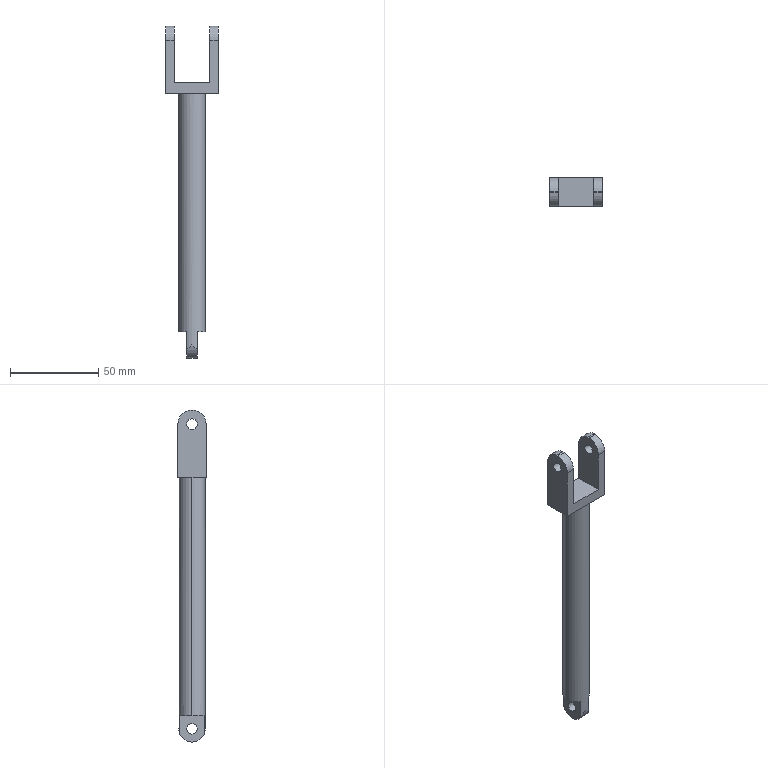Part | SolidWorks | features ICE 5, Extrusion 1 | 1 solid | 27 faces | box 30 x 16 x 188 mm | volume 32315 mm3 | plane 14 | cylinder 13 | commonest cylinder face diameters 6 x6 16 x4 15 x3
STEP:
#1=CARTESIAN_POINT('',(3.,0.,4.5));
#2=VERTEX_POINT('',#1);
#3=CARTESIAN_POINT('',(3.,0.,10.5));
#4=VERTEX_POINT('',#3);
#5=CARTESIAN_POINT('',(3.,0.,7.5));
#6=DIRECTION('',(-1.,0.,0.));
#7=DIRECTION('',(0.,0.,1.));
#8=AXIS2_PLACEMENT_3D('',#5,#6,#7);
#9=CIRCLE('',#8,3.);
#10=EDGE_CURVE('',#2,#4,#9,.T.);
#11=ORIENTED_EDGE('',*,*,#10,.F.);
#12=CARTESIAN_POINT('',(-3.,0.,4.5));
#13=VERTEX_POINT('',#12);
#14=CARTESIAN_POINT('',(15.001,0.,4.5));
#15=DIRECTION('',(-1.,0.,0.));
#16=VECTOR('',#15,1000.);
#17=LINE('',#14,#16);
#18=EDGE_CURVE('',#2,#13,#17,.T.);
#19=ORIENTED_EDGE('',*,*,#18,.T.);
#20=CARTESIAN_POINT('',(-3.,0.,10.5));
#21=VERTEX_POINT('',#20);
#22=CARTESIAN_POINT('',(-3.,0.,7.5));
#23=DIRECTION('',(1.,0.,0.));
#24=DIRECTION('',(0.,0.,-1.));
#25=AXIS2_PLACEMENT_3D('',#22,#23,#24);
#26=CIRCLE('',#25,3.);
#27=EDGE_CURVE('',#21,#13,#26,.T.);
#28=ORIENTED_EDGE('',*,*,#27,.F.);
#29=CARTESIAN_POINT('',(15.001,0.,10.5));
#30=DIRECTION('',(-1.,0.,0.));
#31=VECTOR('',#30,1000.);
#32=LINE('',#29,#31);
#33=EDGE_CURVE('',#4,#21,#32,.T.);
#34=ORIENTED_EDGE('',*,*,#33,.F.);
#35=EDGE_LOOP('',(#11,#19,#28,#34));
#36=FACE_OUTER_BOUND('',#35,.T.);
#37=CARTESIAN_POINT('',(15.001,0.,7.5));
#38=DIRECTION('',(-1.,0.,0.));
#39=DIRECTION('',(0.,0.,1.));
#40=AXIS2_PLACEMENT_3D('',#37,#38,#39);
#41=CYLINDRICAL_SURFACE('',#40,3.);
#42=ADVANCED_FACE('',(#36),#41,.F.);
#43=CARTESIAN_POINT('',(10.,-3.,180.015));
#44=VERTEX_POINT('',#43);
#45=CARTESIAN_POINT('',(10.,3.,180.015));
#46=VERTEX_POINT('',#45);
#47=CARTESIAN_POINT('',(10.,0.,180.015));
#48=DIRECTION('',(1.,0.,0.));
#49=DIRECTION('',(0.,1.,0.));
#50=AXIS2_PLACEMENT_3D('',#47,#48,#49);
#51=CIRCLE('',#50,3.);
#52=EDGE_CURVE('',#44,#46,#51,.T.);
#53=ORIENTED_EDGE('',*,*,#52,.F.);
#54=CARTESIAN_POINT('',(15.,-3.,180.015));
#55=VERTEX_POINT('',#54);
#56=CARTESIAN_POINT('',(-15.,-3.,180.015));
#57=DIRECTION('',(1.,0.,0.));
#58=VECTOR('',#57,1000.);
#59=LINE('',#56,#58);
#60=EDGE_CURVE('',#44,#55,#59,.T.);
#61=ORIENTED_EDGE('',*,*,#60,.T.);
#62=CARTESIAN_POINT('',(15.,3.,180.015));
#63=VERTEX_POINT('',#62);
#64=CARTESIAN_POINT('',(15.,0.,180.015));
#65=DIRECTION('',(-1.,0.,0.));
#66=DIRECTION('',(0.,-1.,0.));
#67=AXIS2_PLACEMENT_3D('',#64,#65,#66);
#68=CIRCLE('',#67,3.);
#69=EDGE_CURVE('',#63,#55,#68,.T.);
#70=ORIENTED_EDGE('',*,*,#69,.F.);
#71=CARTESIAN_POINT('',(-15.,3.,180.015));
#72=DIRECTION('',(1.,0.,0.));
#73=VECTOR('',#72,1000.);
#74=LINE('',#71,#73);
#75=EDGE_CURVE('',#46,#63,#74,.T.);
#76=ORIENTED_EDGE('',*,*,#75,.F.);
#77=EDGE_LOOP('',(#53,#61,#70,#76));
#78=FACE_OUTER_BOUND('',#77,.T.);
#79=CARTESIAN_POINT('',(-15.,0.,180.015));
#80=DIRECTION('',(1.,0.,0.));
#81=DIRECTION('',(0.,1.,0.));
#82=AXIS2_PLACEMENT_3D('',#79,#80,#81);
#83=CYLINDRICAL_SURFACE('',#82,3.);
#84=ADVANCED_FACE('',(#78),#83,.F.);
#85=CARTESIAN_POINT('',(-15.,-3.,180.015));
#86=VERTEX_POINT('',#85);
#87=CARTESIAN_POINT('',(-15.,3.,180.015));
#88=VERTEX_POINT('',#87);
#89=CARTESIAN_POINT('',(-15.,0.,180.015));
#90=DIRECTION('',(1.,0.,0.));
#91=DIRECTION('',(0.,1.,0.));
#92=AXIS2_PLACEMENT_3D('',#89,#90,#91);
#93=CIRCLE('',#92,3.);
#94=EDGE_CURVE('',#86,#88,#93,.T.);
#95=ORIENTED_EDGE('',*,*,#94,.F.);
#96=CARTESIAN_POINT('',(-10.,-3.,180.015));
#97=VERTEX_POINT('',#96);
#98=CARTESIAN_POINT('',(-15.,-3.,180.015));
#99=DIRECTION('',(1.,0.,0.));
#100=VECTOR('',#99,1000.);
#101=LINE('',#98,#100);
#102=EDGE_CURVE('',#86,#97,#101,.T.);
#103=ORIENTED_EDGE('',*,*,#102,.T.);
#104=CARTESIAN_POINT('',(-10.,3.,180.015));
#105=VERTEX_POINT('',#104);
#106=CARTESIAN_POINT('',(-10.,0.,180.015));
#107=DIRECTION('',(-1.,0.,0.));
#108=DIRECTION('',(0.,-1.,0.));
#109=AXIS2_PLACEMENT_3D('',#106,#107,#108);
#110=CIRCLE('',#109,3.);
#111=EDGE_CURVE('',#105,#97,#110,.T.);
#112=ORIENTED_EDGE('',*,*,#111,.F.);
#113=CARTESIAN_POINT('',(-15.,3.,180.015));
#114=DIRECTION('',(1.,0.,0.));
#115=VECTOR('',#114,1000.);
#116=LINE('',#113,#115);
#117=EDGE_CURVE('',#88,#105,#116,.T.);
#118=ORIENTED_EDGE('',*,*,#117,.F.);
#119=EDGE_LOOP('',(#95,#103,#112,#118));
#120=FACE_OUTER_BOUND('',#119,.T.);
#121=CARTESIAN_POINT('',(-15.,0.,180.015));
#122=DIRECTION('',(1.,0.,0.));
#123=DIRECTION('',(0.,1.,0.));
#124=AXIS2_PLACEMENT_3D('',#121,#122,#123);
#125=CYLINDRICAL_SURFACE('',#124,3.);
#126=ADVANCED_FACE('',(#120),#125,.F.);
#127=CARTESIAN_POINT('',(7.5,0.,150.));
#128=VERTEX_POINT('',#127);
#129=CARTESIAN_POINT('',(-7.5,0.,150.));
#130=VERTEX_POINT('',#129);
#131=CARTESIAN_POINT('',(0.,0.,150.));
#132=DIRECTION('',(0.,0.,1.));
#133=DIRECTION('',(1.,0.,0.));
#134=AXIS2_PLACEMENT_3D('',#131,#132,#133);
#135=CIRCLE('',#134,7.5);
#136=EDGE_CURVE('',#128,#130,#135,.T.);
#137=ORIENTED_EDGE('',*,*,#136,.F.);
#138=CARTESIAN_POINT('',(7.5,0.,15.));
#139=VERTEX_POINT('',#138);
#140=CARTESIAN_POINT('',(7.5,0.,150.));
#141=DIRECTION('',(0.,0.,-1.));
#142=VECTOR('',#141,1000.);
#143=LINE('',#140,#142);
#144=EDGE_CURVE('',#128,#139,#143,.T.);
#145=ORIENTED_EDGE('',*,*,#144,.T.);
#146=CARTESIAN_POINT('',(3.,6.874,15.));
#147=VERTEX_POINT('',#146);
#148=CARTESIAN_POINT('',(0.,0.,15.));
#149=DIRECTION('',(0.,0.,1.));
#150=DIRECTION('',(1.,0.,0.));
#151=AXIS2_PLACEMENT_3D('',#148,#149,#150);
#152=CIRCLE('',#151,7.5);
#153=EDGE_CURVE('',#139,#147,#152,.T.);
#154=ORIENTED_EDGE('',*,*,#153,.T.);
#155=CARTESIAN_POINT('',(3.,6.874,4.5));
#156=VERTEX_POINT('',#155);
#157=CARTESIAN_POINT('',(3.,6.874,150.));
#158=DIRECTION('',(0.,0.,-1.));
#159=VECTOR('',#158,1000.);
#160=LINE('',#157,#159);
#161=EDGE_CURVE('',#147,#156,#160,.T.);
#162=ORIENTED_EDGE('',*,*,#161,.T.);
#163=CARTESIAN_POINT('',(0.,7.5,7.5));
#164=VERTEX_POINT('',#163);
#165=CARTESIAN_POINT('',(3.,6.874,4.5));
#166=CARTESIAN_POINT('',(2.05,7.288,5.45));
#167=CARTESIAN_POINT('',(1.036,7.5,6.464));
#168=CARTESIAN_POINT('',(0.,7.5,7.5));
#169=(BOUNDED_CURVE()B_SPLINE_CURVE(3,(#165,#166,#167,#168),.UNSPECIFIED.,.F.,.T.)B_SPLINE_CURVE_WITH_KNOTS((4,4),(1.159,1.571),.UNSPECIFIED.)CURVE()GEOMETRIC_REPRESENTATION_ITEM()RATIONAL_B_SPLINE_CURVE((1.,0.9859,0.9859,1.))REPRESENTATION_ITEM(''));
#170=EDGE_CURVE('',#156,#164,#169,.T.);
#171=ORIENTED_EDGE('',*,*,#170,.T.);
#172=CARTESIAN_POINT('',(-3.,6.874,4.5));
#173=VERTEX_POINT('',#172);
#174=CARTESIAN_POINT('',(0.,7.5,7.5));
#175=CARTESIAN_POINT('',(-1.036,7.5,6.464));
#176=CARTESIAN_POINT('',(-2.05,7.288,5.45));
#177=CARTESIAN_POINT('',(-3.,6.874,4.5));
#178=(BOUNDED_CURVE()B_SPLINE_CURVE(3,(#174,#175,#176,#177),.UNSPECIFIED.,.F.,.T.)B_SPLINE_CURVE_WITH_KNOTS((4,4),(4.712,5.124),.UNSPECIFIED.)CURVE()GEOMETRIC_REPRESENTATION_ITEM()RATIONAL_B_SPLINE_CURVE((1.,0.9859,0.9859,1.))REPRESENTATION_ITEM(''));
#179=EDGE_CURVE('',#164,#173,#178,.T.);
#180=ORIENTED_EDGE('',*,*,#179,.T.);
#181=CARTESIAN_POINT('',(-3.,6.874,15.));
#182=VERTEX_POINT('',#181);
#183=CARTESIAN_POINT('',(-3.,6.874,150.));
#184=DIRECTION('',(0.,0.,1.));
#185=VECTOR('',#184,1000.);
#186=LINE('',#183,#185);
#187=EDGE_CURVE('',#173,#182,#186,.T.);
#188=ORIENTED_EDGE('',*,*,#187,.T.);
#189=CARTESIAN_POINT('',(-7.5,0.,15.));
#190=VERTEX_POINT('',#189);
#191=CARTESIAN_POINT('',(0.,0.,15.));
#192=DIRECTION('',(0.,0.,1.));
#193=DIRECTION('',(1.,0.,0.));
#194=AXIS2_PLACEMENT_3D('',#191,#192,#193);
#195=CIRCLE('',#194,7.5);
#196=EDGE_CURVE('',#182,#190,#195,.T.);
#197=ORIENTED_EDGE('',*,*,#196,.T.);
#198=CARTESIAN_POINT('',(-7.5,0.,150.));
#199=DIRECTION('',(0.,0.,-1.));
#200=VECTOR('',#199,1000.);
#201=LINE('',#198,#200);
#202=EDGE_CURVE('',#130,#190,#201,.T.);
#203=ORIENTED_EDGE('',*,*,#202,.F.);
#204=EDGE_LOOP('',(#137,#145,#154,#162,#171,#180,#188,#197,#203));
#205=FACE_OUTER_BOUND('',#204,.T.);
#206=CARTESIAN_POINT('',(0.,0.,150.));
#207=DIRECTION('',(0.,0.,-1.));
#208=DIRECTION('',(-1.,0.,0.));
#209=AXIS2_PLACEMENT_3D('',#206,#207,#208);
#210=CYLINDRICAL_SURFACE('',#209,7.5);
#211=ADVANCED_FACE('',(#205),#210,.T.);
#212=CARTESIAN_POINT('',(15.,-0.4894,188.));
#213=VERTEX_POINT('',#212);
#214=CARTESIAN_POINT('',(10.,-0.4894,188.));
#215=VERTEX_POINT('',#214);
#216=CARTESIAN_POINT('',(-15.,-0.4894,188.));
#217=DIRECTION('',(-1.,0.,0.));
#218=VECTOR('',#217,1000.);
#219=LINE('',#216,#218);
#220=EDGE_CURVE('',#213,#215,#219,.T.);
#221=ORIENTED_EDGE('',*,*,#220,.F.);
#222=CARTESIAN_POINT('',(15.,0.4894,188.));
#223=VERTEX_POINT('',#222);
#224=CARTESIAN_POINT('',(15.,8.,188.));
#225=DIRECTION('',(0.,1.,0.));
#226=VECTOR('',#225,1000.);
#227=LINE('',#224,#226);
#228=EDGE_CURVE('',#213,#223,#227,.T.);
#229=ORIENTED_EDGE('',*,*,#228,.T.);
#230=CARTESIAN_POINT('',(10.,0.4894,188.));
#231=VERTEX_POINT('',#230);
#232=CARTESIAN_POINT('',(-15.,0.4894,188.));
#233=DIRECTION('',(1.,0.,0.));
#234=VECTOR('',#233,1000.);
#235=LINE('',#232,#234);
#236=EDGE_CURVE('',#231,#223,#235,.T.);
#237=ORIENTED_EDGE('',*,*,#236,.F.);
#238=CARTESIAN_POINT('',(10.,0.,188.));
#239=DIRECTION('',(0.,1.,0.));
#240=VECTOR('',#239,1000.);
#241=LINE('',#238,#240);
#242=EDGE_CURVE('',#215,#231,#241,.T.);
#243=ORIENTED_EDGE('',*,*,#242,.F.);
#244=EDGE_LOOP('',(#221,#229,#237,#243));
#245=FACE_OUTER_BOUND('',#244,.T.);
#246=CARTESIAN_POINT('',(0.,0.,188.));
#247=DIRECTION('',(0.,0.,1.));
#248=DIRECTION('',(1.,0.,0.));
#249=AXIS2_PLACEMENT_3D('',#246,#247,#248);
#250=PLANE('',#249);
#251=ADVANCED_FACE('',(#245),#250,.T.);
#252=ORIENTED_EDGE('',*,*,#144,.F.);
#253=CARTESIAN_POINT('',(0.,0.,150.));
#254=DIRECTION('',(0.,0.,1.));
#255=DIRECTION('',(1.,0.,0.));
#256=AXIS2_PLACEMENT_3D('',#253,#254,#255);
#257=CIRCLE('',#256,7.5);
#258=EDGE_CURVE('',#130,#128,#257,.T.);
#259=ORIENTED_EDGE('',*,*,#258,.F.);
#260=ORIENTED_EDGE('',*,*,#202,.T.);
#261=CARTESIAN_POINT('',(-3.,-6.874,15.));
#262=VERTEX_POINT('',#261);
#263=CARTESIAN_POINT('',(0.,0.,15.));
#264=DIRECTION('',(0.,0.,1.));
#265=DIRECTION('',(1.,0.,0.));
#266=AXIS2_PLACEMENT_3D('',#263,#264,#265);
#267=CIRCLE('',#266,7.5);
#268=EDGE_CURVE('',#190,#262,#267,.T.);
#269=ORIENTED_EDGE('',*,*,#268,.T.);
#270=CARTESIAN_POINT('',(-3.,-6.874,4.5));
#271=VERTEX_POINT('',#270);
#272=CARTESIAN_POINT('',(-3.,-6.874,150.));
#273=DIRECTION('',(0.,0.,-1.));
#274=VECTOR('',#273,1000.);
#275=LINE('',#272,#274);
#276=EDGE_CURVE('',#262,#271,#275,.T.);
#277=ORIENTED_EDGE('',*,*,#276,.T.);
#278=CARTESIAN_POINT('',(0.,-7.5,7.5));
#279=VERTEX_POINT('',#278);
#280=CARTESIAN_POINT('',(-3.,-6.874,4.5));
#281=CARTESIAN_POINT('',(-2.05,-7.288,5.45));
#282=CARTESIAN_POINT('',(-1.036,-7.5,6.464));
#283=CARTESIAN_POINT('',(0.,-7.5,7.5));
#284=(BOUNDED_CURVE()B_SPLINE_CURVE(3,(#280,#281,#282,#283),.UNSPECIFIED.,.F.,.T.)B_SPLINE_CURVE_WITH_KNOTS((4,4),(1.159,1.571),.UNSPECIFIED.)CURVE()GEOMETRIC_REPRESENTATION_ITEM()RATIONAL_B_SPLINE_CURVE((1.,0.9859,0.9859,1.))REPRESENTATION_ITEM(''));
#285=EDGE_CURVE('',#271,#279,#284,.T.);
#286=ORIENTED_EDGE('',*,*,#285,.T.);
#287=CARTESIAN_POINT('',(3.,-6.874,4.5));
#288=VERTEX_POINT('',#287);
#289=CARTESIAN_POINT('',(0.,-7.5,7.5));
#290=CARTESIAN_POINT('',(1.036,-7.5,6.464));
#291=CARTESIAN_POINT('',(2.05,-7.288,5.45));
#292=CARTESIAN_POINT('',(3.,-6.874,4.5));
#293=(BOUNDED_CURVE()B_SPLINE_CURVE(3,(#289,#290,#291,#292),.UNSPECIFIED.,.F.,.T.)B_SPLINE_CURVE_WITH_KNOTS((4,4),(4.712,5.124),.UNSPECIFIED.)CURVE()GEOMETRIC_REPRESENTATION_ITEM()RATIONAL_B_SPLINE_CURVE((1.,0.9859,0.9859,1.))REPRESENTATION_ITEM(''));
#294=EDGE_CURVE('',#279,#288,#293,.T.);
#295=ORIENTED_EDGE('',*,*,#294,.T.);
#296=CARTESIAN_POINT('',(3.,-6.874,15.));
#297=VERTEX_POINT('',#296);
#298=CARTESIAN_POINT('',(3.,-6.874,150.));
#299=DIRECTION('',(0.,0.,1.));
#300=VECTOR('',#299,1000.);
#301=LINE('',#298,#300);
#302=EDGE_CURVE('',#288,#297,#301,.T.);
#303=ORIENTED_EDGE('',*,*,#302,.T.);
#304=CARTESIAN_POINT('',(0.,0.,15.));
#305=DIRECTION('',(0.,0.,1.));
#306=DIRECTION('',(1.,0.,0.));
#307=AXIS2_PLACEMENT_3D('',#304,#305,#306);
#308=CIRCLE('',#307,7.5);
#309=EDGE_CURVE('',#297,#139,#308,.T.);
#310=ORIENTED_EDGE('',*,*,#309,.T.);
#311=EDGE_LOOP('',(#252,#259,#260,#269,#277,#286,#295,#303,#310));
#312=FACE_OUTER_BOUND('',#311,.T.);
#313=CARTESIAN_POINT('',(0.,0.,150.));
#314=DIRECTION('',(0.,0.,-1.));
#315=DIRECTION('',(-1.,0.,0.));
#316=AXIS2_PLACEMENT_3D('',#313,#314,#315);
#317=CYLINDRICAL_SURFACE('',#316,7.5);
#318=ADVANCED_FACE('',(#312),#317,.T.);
#319=ORIENTED_EDGE('',*,*,#69,.T.);
#320=CARTESIAN_POINT('',(15.,0.,180.015));
#321=DIRECTION('',(-1.,0.,0.));
#322=DIRECTION('',(0.,-1.,0.));
#323=AXIS2_PLACEMENT_3D('',#320,#321,#322);
#324=CIRCLE('',#323,3.);
#325=EDGE_CURVE('',#55,#63,#324,.T.);
#326=ORIENTED_EDGE('',*,*,#325,.T.);
#327=EDGE_LOOP('',(#319,#326));
#328=FACE_BOUND('',#327,.T.);
#329=CARTESIAN_POINT('',(15.,8.,180.015));
#330=VERTEX_POINT('',#329);
#331=CARTESIAN_POINT('',(15.,8.,150.));
#332=VERTEX_POINT('',#331);
#333=CARTESIAN_POINT('',(15.,8.,188.));
#334=DIRECTION('',(0.,0.,-1.));
#335=VECTOR('',#334,1000.);
#336=LINE('',#333,#335);
#337=EDGE_CURVE('',#330,#332,#336,.T.);
#338=ORIENTED_EDGE('',*,*,#337,.F.);
#339=CARTESIAN_POINT('',(15.,0.,180.015));
#340=DIRECTION('',(1.,0.,0.));
#341=DIRECTION('',(0.,-1.,0.));
#342=AXIS2_PLACEMENT_3D('',#339,#340,#341);
#343=CIRCLE('',#342,8.);
#344=EDGE_CURVE('',#330,#223,#343,.T.);
#345=ORIENTED_EDGE('',*,*,#344,.T.);
#346=ORIENTED_EDGE('',*,*,#228,.F.);
#347=CARTESIAN_POINT('',(15.,-8.,180.015));
#348=VERTEX_POINT('',#347);
#349=CARTESIAN_POINT('',(15.,0.,180.015));
#350=DIRECTION('',(1.,0.,0.));
#351=DIRECTION('',(0.,-1.,0.));
#352=AXIS2_PLACEMENT_3D('',#349,#350,#351);
#353=CIRCLE('',#352,8.);
#354=EDGE_CURVE('',#213,#348,#353,.T.);
#355=ORIENTED_EDGE('',*,*,#354,.T.);
#356=CARTESIAN_POINT('',(15.,-8.,150.));
#357=VERTEX_POINT('',#356);
#358=CARTESIAN_POINT('',(15.,-8.,188.));
#359=DIRECTION('',(0.,0.,-1.));
#360=VECTOR('',#359,1000.);
#361=LINE('',#358,#360);
#362=EDGE_CURVE('',#348,#357,#361,.T.);
#363=ORIENTED_EDGE('',*,*,#362,.T.);
#364=CARTESIAN_POINT('',(15.,8.,150.));
#365=DIRECTION('',(0.,1.,0.));
#366=VECTOR('',#365,1000.);
#367=LINE('',#364,#366);
#368=EDGE_CURVE('',#357,#332,#367,.T.);
#369=ORIENTED_EDGE('',*,*,#368,.T.);
#370=EDGE_LOOP('',(#338,#345,#346,#355,#363,#369));
#371=FACE_OUTER_BOUND('',#370,.T.);
#372=CARTESIAN_POINT('',(15.,8.,188.));
#373=DIRECTION('',(-1.,0.,0.));
#374=DIRECTION('',(0.,-1.,0.));
#375=AXIS2_PLACEMENT_3D('',#372,#373,#374);
#376=PLANE('',#375);
#377=ADVANCED_FACE('',(#328,#371),#376,.F.);
#378=CARTESIAN_POINT('',(-15.,8.,180.015));
#379=VERTEX_POINT('',#378);
#380=CARTESIAN_POINT('',(-15.,8.,150.));
#381=VERTEX_POINT('',#380);
#382=CARTESIAN_POINT('',(-15.,8.,188.));
#383=DIRECTION('',(0.,0.,-1.));
#384=VECTOR('',#383,1000.);
#385=LINE('',#382,#384);
#386=EDGE_CURVE('',#379,#381,#385,.T.);
#387=ORIENTED_EDGE('',*,*,#386,.F.);
#388=CARTESIAN_POINT('',(-10.,8.,180.015));
#389=VERTEX_POINT('',#388);
#390=CARTESIAN_POINT('',(-15.,8.,180.015));
#391=DIRECTION('',(1.,0.,0.));
#392=VECTOR('',#391,1000.);
#393=LINE('',#390,#392);
#394=EDGE_CURVE('',#379,#389,#393,.T.);
#395=ORIENTED_EDGE('',*,*,#394,.T.);
#396=CARTESIAN_POINT('',(-10.,8.,156.));
#397=VERTEX_POINT('',#396);
#398=CARTESIAN_POINT('',(-10.,8.,188.));
#399=DIRECTION('',(0.,0.,-1.));
#400=VECTOR('',#399,1000.);
#401=LINE('',#398,#400);
#402=EDGE_CURVE('',#389,#397,#401,.T.);
#403=ORIENTED_EDGE('',*,*,#402,.T.);
#404=CARTESIAN_POINT('',(10.,8.,156.));
#405=VERTEX_POINT('',#404);
#406=CARTESIAN_POINT('',(-15.,8.,156.));
#407=DIRECTION('',(-1.,0.,0.));
#408=VECTOR('',#407,1000.);
#409=LINE('',#406,#408);
#410=EDGE_CURVE('',#405,#397,#409,.T.);
#411=ORIENTED_EDGE('',*,*,#410,.F.);
#412=CARTESIAN_POINT('',(10.,8.,180.015));
#413=VERTEX_POINT('',#412);
#414=CARTESIAN_POINT('',(10.,8.,188.));
#415=DIRECTION('',(0.,0.,1.));
#416=VECTOR('',#415,1000.);
#417=LINE('',#414,#416);
#418=EDGE_CURVE('',#405,#413,#417,.T.);
#419=ORIENTED_EDGE('',*,*,#418,.T.);
#420=CARTESIAN_POINT('',(-15.,8.,180.015));
#421=DIRECTION('',(1.,0.,0.));
#422=VECTOR('',#421,1000.);
#423=LINE('',#420,#422);
#424=EDGE_CURVE('',#413,#330,#423,.T.);
#425=ORIENTED_EDGE('',*,*,#424,.T.);
#426=ORIENTED_EDGE('',*,*,#337,.T.);
#427=CARTESIAN_POINT('',(-15.,8.,150.));
#428=DIRECTION('',(-1.,0.,0.));
#429=VECTOR('',#428,1000.);
#430=LINE('',#427,#429);
#431=EDGE_CURVE('',#332,#381,#430,.T.);
#432=ORIENTED_EDGE('',*,*,#431,.T.);
#433=EDGE_LOOP('',(#387,#395,#403,#411,#419,#425,#426,#432));
#434=FACE_OUTER_BOUND('',#433,.T.);
#435=CARTESIAN_POINT('',(-15.,8.,188.));
#436=DIRECTION('',(0.,-1.,0.));
#437=DIRECTION('',(0.,0.,-1.));
#438=AXIS2_PLACEMENT_3D('',#435,#436,#437);
#439=PLANE('',#438);
#440=ADVANCED_FACE('',(#434),#439,.F.);
#441=CARTESIAN_POINT('',(-15.,0.,180.015));
#442=DIRECTION('',(1.,0.,0.));
#443=DIRECTION('',(0.,1.,0.));
#444=AXIS2_PLACEMENT_3D('',#441,#442,#443);
#445=CIRCLE('',#444,3.);
#446=EDGE_CURVE('',#88,#86,#445,.T.);
#447=ORIENTED_EDGE('',*,*,#446,.T.);
#448=ORIENTED_EDGE('',*,*,#94,.T.);
#449=EDGE_LOOP('',(#447,#448));
#450=FACE_BOUND('',#449,.T.);
#451=CARTESIAN_POINT('',(-15.,-8.,180.015));
#452=VERTEX_POINT('',#451);
#453=CARTESIAN_POINT('',(-15.,-8.,150.));
#454=VERTEX_POINT('',#453);
#455=CARTESIAN_POINT('',(-15.,-8.,188.));
#456=DIRECTION('',(0.,0.,-1.));
#457=VECTOR('',#456,1000.);
#458=LINE('',#455,#457);
#459=EDGE_CURVE('',#452,#454,#458,.T.);
#460=ORIENTED_EDGE('',*,*,#459,.F.);
#461=CARTESIAN_POINT('',(-15.,-0.4894,188.));
#462=VERTEX_POINT('',#461);
#463=CARTESIAN_POINT('',(-15.,0.,180.015));
#464=DIRECTION('',(-1.,0.,0.));
#465=DIRECTION('',(0.,1.,0.));
#466=AXIS2_PLACEMENT_3D('',#463,#464,#465);
#467=CIRCLE('',#466,8.);
#468=EDGE_CURVE('',#452,#462,#467,.T.);
#469=ORIENTED_EDGE('',*,*,#468,.T.);
#470=CARTESIAN_POINT('',(-15.,0.4894,188.));
#471=VERTEX_POINT('',#470);
#472=CARTESIAN_POINT('',(-15.,8.,188.));
#473=DIRECTION('',(0.,-1.,0.));
#474=VECTOR('',#473,1000.);
#475=LINE('',#472,#474);
#476=EDGE_CURVE('',#471,#462,#475,.T.);
#477=ORIENTED_EDGE('',*,*,#476,.F.);
#478=CARTESIAN_POINT('',(-15.,0.,180.015));
#479=DIRECTION('',(-1.,0.,0.));
#480=DIRECTION('',(0.,1.,0.));
#481=AXIS2_PLACEMENT_3D('',#478,#479,#480);
#482=CIRCLE('',#481,8.);
#483=EDGE_CURVE('',#471,#379,#482,.T.);
#484=ORIENTED_EDGE('',*,*,#483,.T.);
#485=ORIENTED_EDGE('',*,*,#386,.T.);
#486=CARTESIAN_POINT('',(-15.,8.,150.));
#487=DIRECTION('',(0.,-1.,0.));
#488=VECTOR('',#487,1000.);
#489=LINE('',#486,#488);
#490=EDGE_CURVE('',#381,#454,#489,.T.);
#491=ORIENTED_EDGE('',*,*,#490,.T.);
#492=EDGE_LOOP('',(#460,#469,#477,#484,#485,#491));
#493=FACE_OUTER_BOUND('',#492,.T.);
#494=CARTESIAN_POINT('',(-15.,8.,188.));
#495=DIRECTION('',(1.,0.,0.));
#496=DIRECTION('',(0.,1.,0.));
#497=AXIS2_PLACEMENT_3D('',#494,#495,#496);
#498=PLANE('',#497);
#499=ADVANCED_FACE('',(#450,#493),#498,.F.);
#500=ORIENTED_EDGE('',*,*,#362,.F.);
#501=CARTESIAN_POINT('',(10.,-8.,180.015));
#502=VERTEX_POINT('',#501);
#503=CARTESIAN_POINT('',(-15.,-8.,180.015));
#504=DIRECTION('',(1.,0.,0.));
#505=VECTOR('',#504,1000.);
#506=LINE('',#503,#505);
#507=EDGE_CURVE('',#502,#348,#506,.T.);
#508=ORIENTED_EDGE('',*,*,#507,.F.);
#509=CARTESIAN_POINT('',(10.,-8.,156.));
#510=VERTEX_POINT('',#509);
#511=CARTESIAN_POINT('',(10.,-8.,188.));
#512=DIRECTION('',(0.,0.,-1.));
#513=VECTOR('',#512,1000.);
#514=LINE('',#511,#513);
#515=EDGE_CURVE('',#502,#510,#514,.T.);
#516=ORIENTED_EDGE('',*,*,#515,.T.);
#517=CARTESIAN_POINT('',(-10.,-8.,156.));
#518=VERTEX_POINT('',#517);
#519=CARTESIAN_POINT('',(-15.,-8.,156.));
#520=DIRECTION('',(1.,0.,0.));
#521=VECTOR('',#520,1000.);
#522=LINE('',#519,#521);
#523=EDGE_CURVE('',#518,#510,#522,.T.);
#524=ORIENTED_EDGE('',*,*,#523,.F.);
#525=CARTESIAN_POINT('',(-10.,-8.,180.015));
#526=VERTEX_POINT('',#525);
#527=CARTESIAN_POINT('',(-10.,-8.,188.));
#528=DIRECTION('',(0.,0.,1.));
#529=VECTOR('',#528,1000.);
#530=LINE('',#527,#529);
#531=EDGE_CURVE('',#518,#526,#530,.T.);
#532=ORIENTED_EDGE('',*,*,#531,.T.);
#533=CARTESIAN_POINT('',(-15.,-8.,180.015));
#534=DIRECTION('',(1.,0.,0.));
#535=VECTOR('',#534,1000.);
#536=LINE('',#533,#535);
#537=EDGE_CURVE('',#452,#526,#536,.T.);
#538=ORIENTED_EDGE('',*,*,#537,.F.);
#539=ORIENTED_EDGE('',*,*,#459,.T.);
#540=CARTESIAN_POINT('',(-15.,-8.,150.));
#541=DIRECTION('',(1.,0.,0.));
#542=VECTOR('',#541,1000.);
#543=LINE('',#540,#542);
#544=EDGE_CURVE('',#454,#357,#543,.T.);
#545=ORIENTED_EDGE('',*,*,#544,.T.);
#546=EDGE_LOOP('',(#500,#508,#516,#524,#532,#538,#539,#545));
#547=FACE_OUTER_BOUND('',#546,.T.);
#548=CARTESIAN_POINT('',(-15.,-8.,188.));
#549=DIRECTION('',(0.,1.,0.));
#550=DIRECTION('',(0.,0.,1.));
#551=AXIS2_PLACEMENT_3D('',#548,#549,#550);
#552=PLANE('',#551);
#553=ADVANCED_FACE('',(#547),#552,.F.);
#554=CARTESIAN_POINT('',(-10.,-0.4894,188.));
#555=VERTEX_POINT('',#554);
#556=CARTESIAN_POINT('',(-15.,-0.4894,188.));
#557=DIRECTION('',(-1.,0.,0.));
#558=VECTOR('',#557,1000.);
#559=LINE('',#556,#558);
#560=EDGE_CURVE('',#555,#462,#559,.T.);
#561=ORIENTED_EDGE('',*,*,#560,.F.);
#562=CARTESIAN_POINT('',(-10.,0.4894,188.));
#563=VERTEX_POINT('',#562);
#564=CARTESIAN_POINT('',(-10.,0.,188.));
#565=DIRECTION('',(0.,-1.,0.));
#566=VECTOR('',#565,1000.);
#567=LINE('',#564,#566);
#568=EDGE_CURVE('',#563,#555,#567,.T.);
#569=ORIENTED_EDGE('',*,*,#568,.F.);
#570=CARTESIAN_POINT('',(-15.,0.4894,188.));
#571=DIRECTION('',(1.,0.,0.));
#572=VECTOR('',#571,1000.);
#573=LINE('',#570,#572);
#574=EDGE_CURVE('',#471,#563,#573,.T.);
#575=ORIENTED_EDGE('',*,*,#574,.F.);
#576=ORIENTED_EDGE('',*,*,#476,.T.);
#577=EDGE_LOOP('',(#561,#569,#575,#576));
#578=FACE_OUTER_BOUND('',#577,.T.);
#579=CARTESIAN_POINT('',(0.,0.,188.));
#580=DIRECTION('',(0.,0.,1.));
#581=DIRECTION('',(1.,0.,0.));
#582=AXIS2_PLACEMENT_3D('',#579,#580,#581);
#583=PLANE('',#582);
#584=ADVANCED_FACE('',(#578),#583,.T.);
#585=ORIENTED_EDGE('',*,*,#258,.T.);
#586=ORIENTED_EDGE('',*,*,#136,.T.);
#587=EDGE_LOOP('',(#585,#586));
#588=FACE_BOUND('',#587,.T.);
#589=ORIENTED_EDGE('',*,*,#368,.F.);
#590=ORIENTED_EDGE('',*,*,#544,.F.);
#591=ORIENTED_EDGE('',*,*,#490,.F.);
#592=ORIENTED_EDGE('',*,*,#431,.F.);
#593=EDGE_LOOP('',(#589,#590,#591,#592));
#594=FACE_OUTER_BOUND('',#593,.T.);
#595=CARTESIAN_POINT('',(0.,0.,150.));
#596=DIRECTION('',(0.,0.,1.));
#597=DIRECTION('',(1.,0.,0.));
#598=AXIS2_PLACEMENT_3D('',#595,#596,#597);
#599=PLANE('',#598);
#600=ADVANCED_FACE('',(#588,#594),#599,.F.);
#601=ORIENTED_EDGE('',*,*,#410,.T.);
#602=CARTESIAN_POINT('',(-10.,9.679,156.));
#603=DIRECTION('',(0.,-1.,0.));
#604=VECTOR('',#603,1000.);
#605=LINE('',#602,#604);
#606=EDGE_CURVE('',#397,#518,#605,.T.);
#607=ORIENTED_EDGE('',*,*,#606,.T.);
#608=ORIENTED_EDGE('',*,*,#523,.T.);
#609=CARTESIAN_POINT('',(10.,9.679,156.));
#610=DIRECTION('',(0.,1.,0.));
#611=VECTOR('',#610,1000.);
#612=LINE('',#609,#611);
#613=EDGE_CURVE('',#510,#405,#612,.T.);
#614=ORIENTED_EDGE('',*,*,#613,.T.);
#615=EDGE_LOOP('',(#601,#607,#608,#614));
#616=FACE_OUTER_BOUND('',#615,.T.);
#617=CARTESIAN_POINT('',(0.,0.,156.));
#618=DIRECTION('',(0.,0.,1.));
#619=DIRECTION('',(1.,0.,0.));
#620=AXIS2_PLACEMENT_3D('',#617,#618,#619);
#621=PLANE('',#620);
#622=ADVANCED_FACE('',(#616),#621,.T.);
#623=CARTESIAN_POINT('',(10.,0.,180.015));
#624=DIRECTION('',(1.,0.,0.));
#625=DIRECTION('',(0.,1.,0.));
#626=AXIS2_PLACEMENT_3D('',#623,#624,#625);
#627=CIRCLE('',#626,3.);
#628=EDGE_CURVE('',#46,#44,#627,.T.);
#629=ORIENTED_EDGE('',*,*,#628,.T.);
#630=ORIENTED_EDGE('',*,*,#52,.T.);
#631=EDGE_LOOP('',(#629,#630));
#632=FACE_BOUND('',#631,.T.);
#633=ORIENTED_EDGE('',*,*,#515,.F.);
#634=CARTESIAN_POINT('',(10.,0.,180.015));
#635=DIRECTION('',(-1.,0.,0.));
#636=DIRECTION('',(0.,1.,0.));
#637=AXIS2_PLACEMENT_3D('',#634,#635,#636);
#638=CIRCLE('',#637,8.);
#639=EDGE_CURVE('',#502,#215,#638,.T.);
#640=ORIENTED_EDGE('',*,*,#639,.T.);
#641=ORIENTED_EDGE('',*,*,#242,.T.);
#642=CARTESIAN_POINT('',(10.,0.,180.015));
#643=DIRECTION('',(-1.,0.,0.));
#644=DIRECTION('',(0.,1.,0.));
#645=AXIS2_PLACEMENT_3D('',#642,#643,#644);
#646=CIRCLE('',#645,8.);
#647=EDGE_CURVE('',#231,#413,#646,.T.);
#648=ORIENTED_EDGE('',*,*,#647,.T.);
#649=ORIENTED_EDGE('',*,*,#418,.F.);
#650=ORIENTED_EDGE('',*,*,#613,.F.);
#651=EDGE_LOOP('',(#633,#640,#641,#648,#649,#650));
#652=FACE_OUTER_BOUND('',#651,.T.);
#653=CARTESIAN_POINT('',(10.,9.679,156.));
#654=DIRECTION('',(1.,0.,0.));
#655=DIRECTION('',(0.,1.,0.));
#656=AXIS2_PLACEMENT_3D('',#653,#654,#655);
#657=PLANE('',#656);
#658=ADVANCED_FACE('',(#632,#652),#657,.F.);
#659=ORIENTED_EDGE('',*,*,#111,.T.);
#660=CARTESIAN_POINT('',(-10.,0.,180.015));
#661=DIRECTION('',(-1.,0.,0.));
#662=DIRECTION('',(0.,-1.,0.));
#663=AXIS2_PLACEMENT_3D('',#660,#661,#662);
#664=CIRCLE('',#663,3.);
#665=EDGE_CURVE('',#97,#105,#664,.T.);
#666=ORIENTED_EDGE('',*,*,#665,.T.);
#667=EDGE_LOOP('',(#659,#666));
#668=FACE_BOUND('',#667,.T.);
#669=ORIENTED_EDGE('',*,*,#402,.F.);
#670=CARTESIAN_POINT('',(-10.,0.,180.015));
#671=DIRECTION('',(1.,0.,0.));
#672=DIRECTION('',(0.,-1.,0.));
#673=AXIS2_PLACEMENT_3D('',#670,#671,#672);
#674=CIRCLE('',#673,8.);
#675=EDGE_CURVE('',#389,#563,#674,.T.);
#676=ORIENTED_EDGE('',*,*,#675,.T.);
#677=ORIENTED_EDGE('',*,*,#568,.T.);
#678=CARTESIAN_POINT('',(-10.,0.,180.015));
#679=DIRECTION('',(1.,0.,0.));
#680=DIRECTION('',(0.,-1.,0.));
#681=AXIS2_PLACEMENT_3D('',#678,#679,#680);
#682=CIRCLE('',#681,8.);
#683=EDGE_CURVE('',#555,#526,#682,.T.);
#684=ORIENTED_EDGE('',*,*,#683,.T.);
#685=ORIENTED_EDGE('',*,*,#531,.F.);
#686=ORIENTED_EDGE('',*,*,#606,.F.);
#687=EDGE_LOOP('',(#669,#676,#677,#684,#685,#686));
#688=FACE_OUTER_BOUND('',#687,.T.);
#689=CARTESIAN_POINT('',(-10.,9.679,156.));
#690=DIRECTION('',(-1.,0.,0.));
#691=DIRECTION('',(0.,-1.,0.));
#692=AXIS2_PLACEMENT_3D('',#689,#690,#691);
#693=PLANE('',#692);
#694=ADVANCED_FACE('',(#668,#688),#693,.F.);
#695=ORIENTED_EDGE('',*,*,#102,.F.);
#696=ORIENTED_EDGE('',*,*,#446,.F.);
#697=ORIENTED_EDGE('',*,*,#117,.T.);
#698=ORIENTED_EDGE('',*,*,#665,.F.);
#699=EDGE_LOOP('',(#695,#696,#697,#698));
#700=FACE_OUTER_BOUND('',#699,.T.);
#701=CARTESIAN_POINT('',(-15.,0.,180.015));
#702=DIRECTION('',(1.,0.,0.));
#703=DIRECTION('',(0.,1.,0.));
#704=AXIS2_PLACEMENT_3D('',#701,#702,#703);
#705=CYLINDRICAL_SURFACE('',#704,3.);
#706=ADVANCED_FACE('',(#700),#705,.F.);
#707=ORIENTED_EDGE('',*,*,#560,.T.);
#708=ORIENTED_EDGE('',*,*,#468,.F.);
#709=ORIENTED_EDGE('',*,*,#537,.T.);
#710=ORIENTED_EDGE('',*,*,#683,.F.);
#711=EDGE_LOOP('',(#707,#708,#709,#710));
#712=FACE_OUTER_BOUND('',#711,.T.);
#713=CARTESIAN_POINT('',(-15.,0.,180.015));
#714=DIRECTION('',(1.,0.,0.));
#715=DIRECTION('',(0.,1.,0.));
#716=AXIS2_PLACEMENT_3D('',#713,#714,#715);
#717=CYLINDRICAL_SURFACE('',#716,8.);
#718=ADVANCED_FACE('',(#712),#717,.T.);
#719=ORIENTED_EDGE('',*,*,#574,.T.);
#720=ORIENTED_EDGE('',*,*,#675,.F.);
#721=ORIENTED_EDGE('',*,*,#394,.F.);
#722=ORIENTED_EDGE('',*,*,#483,.F.);
#723=EDGE_LOOP('',(#719,#720,#721,#722));
#724=FACE_OUTER_BOUND('',#723,.T.);
#725=CARTESIAN_POINT('',(-15.,0.,180.015));
#726=DIRECTION('',(1.,0.,0.));
#727=DIRECTION('',(0.,1.,0.));
#728=AXIS2_PLACEMENT_3D('',#725,#726,#727);
#729=CYLINDRICAL_SURFACE('',#728,8.);
#730=ADVANCED_FACE('',(#724),#729,.T.);
#731=ORIENTED_EDGE('',*,*,#60,.F.);
#732=ORIENTED_EDGE('',*,*,#628,.F.);
#733=ORIENTED_EDGE('',*,*,#75,.T.);
#734=ORIENTED_EDGE('',*,*,#325,.F.);
#735=EDGE_LOOP('',(#731,#732,#733,#734));
#736=FACE_OUTER_BOUND('',#735,.T.);
#737=CARTESIAN_POINT('',(-15.,0.,180.015));
#738=DIRECTION('',(1.,0.,0.));
#739=DIRECTION('',(0.,1.,0.));
#740=AXIS2_PLACEMENT_3D('',#737,#738,#739);
#741=CYLINDRICAL_SURFACE('',#740,3.);
#742=ADVANCED_FACE('',(#736),#741,.F.);
#743=ORIENTED_EDGE('',*,*,#424,.F.);
#744=ORIENTED_EDGE('',*,*,#647,.F.);
#745=ORIENTED_EDGE('',*,*,#236,.T.);
#746=ORIENTED_EDGE('',*,*,#344,.F.);
#747=EDGE_LOOP('',(#743,#744,#745,#746));
#748=FACE_OUTER_BOUND('',#747,.T.);
#749=CARTESIAN_POINT('',(-15.,0.,180.015));
#750=DIRECTION('',(1.,0.,0.));
#751=DIRECTION('',(0.,1.,0.));
#752=AXIS2_PLACEMENT_3D('',#749,#750,#751);
#753=CYLINDRICAL_SURFACE('',#752,8.);
#754=ADVANCED_FACE('',(#748),#753,.T.);
#755=ORIENTED_EDGE('',*,*,#220,.T.);
#756=ORIENTED_EDGE('',*,*,#639,.F.);
#757=ORIENTED_EDGE('',*,*,#507,.T.);
#758=ORIENTED_EDGE('',*,*,#354,.F.);
#759=EDGE_LOOP('',(#755,#756,#757,#758));
#760=FACE_OUTER_BOUND('',#759,.T.);
#761=CARTESIAN_POINT('',(-15.,0.,180.015));
#762=DIRECTION('',(1.,0.,0.));
#763=DIRECTION('',(0.,1.,0.));
#764=AXIS2_PLACEMENT_3D('',#761,#762,#763);
#765=CYLINDRICAL_SURFACE('',#764,8.);
#766=ADVANCED_FACE('',(#760),#765,.T.);
#767=CARTESIAN_POINT('',(3.,-8.001,15.));
#768=DIRECTION('',(0.,1.,0.));
#769=VECTOR('',#768,1000.);
#770=LINE('',#767,#769);
#771=EDGE_CURVE('',#297,#147,#770,.T.);
#772=ORIENTED_EDGE('',*,*,#771,.T.);
#773=ORIENTED_EDGE('',*,*,#153,.F.);
#774=ORIENTED_EDGE('',*,*,#309,.F.);
#775=EDGE_LOOP('',(#772,#773,#774));
#776=FACE_OUTER_BOUND('',#775,.T.);
#777=CARTESIAN_POINT('',(22.943,-8.001,15.));
#778=DIRECTION('',(0.,0.,1.));
#779=DIRECTION('',(1.,0.,0.));
#780=AXIS2_PLACEMENT_3D('',#777,#778,#779);
#781=PLANE('',#780);
#782=ADVANCED_FACE('',(#776),#781,.F.);
#783=CARTESIAN_POINT('',(3.,0.,7.5));
#784=DIRECTION('',(-1.,0.,0.));
#785=DIRECTION('',(0.,0.,1.));
#786=AXIS2_PLACEMENT_3D('',#783,#784,#785);
#787=CIRCLE('',#786,3.);
#788=EDGE_CURVE('',#4,#2,#787,.T.);
#789=ORIENTED_EDGE('',*,*,#788,.T.);
#790=ORIENTED_EDGE('',*,*,#10,.T.);
#791=EDGE_LOOP('',(#789,#790));
#792=FACE_BOUND('',#791,.T.);
#793=ORIENTED_EDGE('',*,*,#302,.F.);
#794=CARTESIAN_POINT('',(3.,0.,7.5));
#795=DIRECTION('',(1.,0.,0.));
#796=DIRECTION('',(0.,0.,1.));
#797=AXIS2_PLACEMENT_3D('',#794,#795,#796);
#798=CIRCLE('',#797,7.5);
#799=EDGE_CURVE('',#288,#156,#798,.T.);
#800=ORIENTED_EDGE('',*,*,#799,.T.);
#801=ORIENTED_EDGE('',*,*,#161,.F.);
#802=ORIENTED_EDGE('',*,*,#771,.F.);
#803=EDGE_LOOP('',(#793,#800,#801,#802));
#804=FACE_OUTER_BOUND('',#803,.T.);
#805=CARTESIAN_POINT('',(3.,-8.001,15.));
#806=DIRECTION('',(-1.,0.,0.));
#807=DIRECTION('',(0.,0.,1.));
#808=AXIS2_PLACEMENT_3D('',#805,#806,#807);
#809=PLANE('',#808);
#810=ADVANCED_FACE('',(#792,#804),#809,.F.);
#811=CARTESIAN_POINT('',(-3.,-8.001,15.));
#812=DIRECTION('',(0.,1.,0.));
#813=VECTOR('',#812,1000.);
#814=LINE('',#811,#813);
#815=EDGE_CURVE('',#262,#182,#814,.T.);
#816=ORIENTED_EDGE('',*,*,#815,.F.);
#817=ORIENTED_EDGE('',*,*,#268,.F.);
#818=ORIENTED_EDGE('',*,*,#196,.F.);
#819=EDGE_LOOP('',(#816,#817,#818));
#820=FACE_OUTER_BOUND('',#819,.T.);
#821=CARTESIAN_POINT('',(-7.5,-8.001,15.));
#822=DIRECTION('',(0.,0.,1.));
#823=DIRECTION('',(1.,0.,0.));
#824=AXIS2_PLACEMENT_3D('',#821,#822,#823);
#825=PLANE('',#824);
#826=ADVANCED_FACE('',(#820),#825,.F.);
#827=ORIENTED_EDGE('',*,*,#27,.T.);
#828=CARTESIAN_POINT('',(-3.,0.,7.5));
#829=DIRECTION('',(1.,0.,0.));
#830=DIRECTION('',(0.,0.,-1.));
#831=AXIS2_PLACEMENT_3D('',#828,#829,#830);
#832=CIRCLE('',#831,3.);
#833=EDGE_CURVE('',#13,#21,#832,.T.);
#834=ORIENTED_EDGE('',*,*,#833,.T.);
#835=EDGE_LOOP('',(#827,#834));
#836=FACE_BOUND('',#835,.T.);
#837=CARTESIAN_POINT('',(-3.,0.,7.5));
#838=DIRECTION('',(-1.,0.,0.));
#839=DIRECTION('',(0.,0.,-1.));
#840=AXIS2_PLACEMENT_3D('',#837,#838,#839);
#841=CIRCLE('',#840,7.5);
#842=EDGE_CURVE('',#173,#271,#841,.T.);
#843=ORIENTED_EDGE('',*,*,#842,.T.);
#844=ORIENTED_EDGE('',*,*,#276,.F.);
#845=ORIENTED_EDGE('',*,*,#815,.T.);
#846=ORIENTED_EDGE('',*,*,#187,.F.);
#847=EDGE_LOOP('',(#843,#844,#845,#846));
#848=FACE_OUTER_BOUND('',#847,.T.);
#849=CARTESIAN_POINT('',(-3.,-8.001,0.));
#850=DIRECTION('',(1.,0.,0.));
#851=DIRECTION('',(0.,0.,-1.));
#852=AXIS2_PLACEMENT_3D('',#849,#850,#851);
#853=PLANE('',#852);
#854=ADVANCED_FACE('',(#836,#848),#853,.F.);
#855=ORIENTED_EDGE('',*,*,#18,.F.);
#856=ORIENTED_EDGE('',*,*,#788,.F.);
#857=ORIENTED_EDGE('',*,*,#33,.T.);
#858=ORIENTED_EDGE('',*,*,#833,.F.);
#859=EDGE_LOOP('',(#855,#856,#857,#858));
#860=FACE_OUTER_BOUND('',#859,.T.);
#861=CARTESIAN_POINT('',(15.001,0.,7.5));
#862=DIRECTION('',(-1.,0.,0.));
#863=DIRECTION('',(0.,0.,1.));
#864=AXIS2_PLACEMENT_3D('',#861,#862,#863);
#865=CYLINDRICAL_SURFACE('',#864,3.);
#866=ADVANCED_FACE('',(#860),#865,.F.);
#867=ORIENTED_EDGE('',*,*,#842,.F.);
#868=ORIENTED_EDGE('',*,*,#179,.F.);
#869=ORIENTED_EDGE('',*,*,#170,.F.);
#870=ORIENTED_EDGE('',*,*,#799,.F.);
#871=ORIENTED_EDGE('',*,*,#294,.F.);
#872=ORIENTED_EDGE('',*,*,#285,.F.);
#873=EDGE_LOOP('',(#867,#868,#869,#870,#871,#872));
#874=FACE_OUTER_BOUND('',#873,.T.);
#875=CARTESIAN_POINT('',(15.001,0.,7.5));
#876=DIRECTION('',(-1.,0.,0.));
#877=DIRECTION('',(0.,0.,1.));
#878=AXIS2_PLACEMENT_3D('',#875,#876,#877);
#879=CYLINDRICAL_SURFACE('',#878,7.5);
#880=ADVANCED_FACE('',(#874),#879,.T.);
#881=CLOSED_SHELL('',(#42,#84,#126,#211,#251,#318,#377,#440,#499,#553,#584,#600,#622,#658,#694,#706,#718,#730,#742,#754,#766,#782,#810,#826,#854,#866,#880));
#882=MANIFOLD_SOLID_BREP('',#881);
#883=CARTESIAN_POINT('',(0.,0.,0.));
#884=DIRECTION('',(0.,0.,1.));
#885=DIRECTION('',(1.,0.,0.));
#886=AXIS2_PLACEMENT_3D('',#883,#884,#885);
#887=(LENGTH_UNIT()NAMED_UNIT(*)SI_UNIT(.MILLI.,.METRE.));
#888=UNCERTAINTY_MEASURE_WITH_UNIT(LENGTH_MEASURE(0.00001),#887,'','');
#889=(NAMED_UNIT(*)PLANE_ANGLE_UNIT()SI_UNIT($,.RADIAN.));
#890=(NAMED_UNIT(*)SI_UNIT($,.STERADIAN.)SOLID_ANGLE_UNIT());
#891=(GEOMETRIC_REPRESENTATION_CONTEXT(3)GLOBAL_UNCERTAINTY_ASSIGNED_CONTEXT((#888))GLOBAL_UNIT_ASSIGNED_CONTEXT((#887,#889,#890))REPRESENTATION_CONTEXT('',''));
#892=ADVANCED_BREP_SHAPE_REPRESENTATION('',(#882,#886),#891);